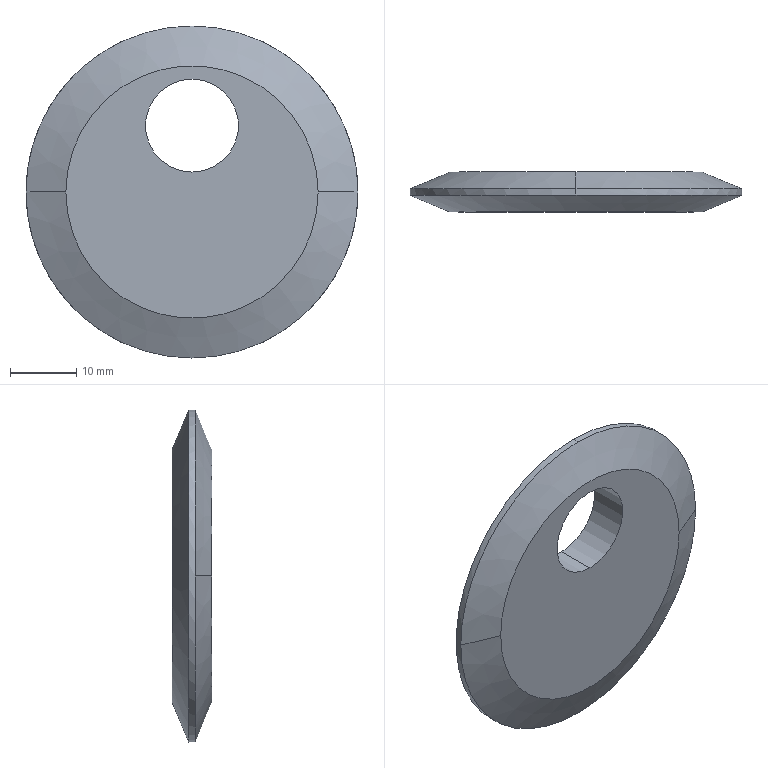Part | SolidWorks | features BaseBody 1 | 1 solid | 10 faces | box 50 x 6 x 50 mm | volume 8690 mm3 | cylinder 4 | cone 4 | plane 2 | commonest cylinder face diameters 14 x2 50 x2
STEP:
#1=CARTESIAN_POINT('',(57.247,561.007,-306.268));
#2=VERTEX_POINT('',#1);
#3=CARTESIAN_POINT('',(57.247,561.007,-292.268));
#4=VERTEX_POINT('',#3);
#5=CARTESIAN_POINT('',(57.247,561.007,-299.268));
#6=DIRECTION('',(0.,1.,0.));
#7=DIRECTION('',(0.,0.,1.));
#8=AXIS2_PLACEMENT_3D('',#5,#6,#7);
#9=CIRCLE('',#8,7.);
#10=EDGE_CURVE('',#2,#4,#9,.T.);
#11=ORIENTED_EDGE('',*,*,#10,.F.);
#12=CARTESIAN_POINT('',(57.247,567.007,-306.268));
#13=VERTEX_POINT('',#12);
#14=CARTESIAN_POINT('',(57.247,458.514,-306.268));
#15=DIRECTION('',(0.,1.,0.));
#16=VECTOR('',#15,1000.);
#17=LINE('',#14,#16);
#18=EDGE_CURVE('',#2,#13,#17,.T.);
#19=ORIENTED_EDGE('',*,*,#18,.T.);
#20=CARTESIAN_POINT('',(57.247,567.007,-292.268));
#21=VERTEX_POINT('',#20);
#22=CARTESIAN_POINT('',(57.247,567.007,-299.268));
#23=DIRECTION('',(0.,-1.,0.));
#24=DIRECTION('',(0.,0.,1.));
#25=AXIS2_PLACEMENT_3D('',#22,#23,#24);
#26=CIRCLE('',#25,7.);
#27=EDGE_CURVE('',#21,#13,#26,.T.);
#28=ORIENTED_EDGE('',*,*,#27,.F.);
#29=CARTESIAN_POINT('',(57.247,458.514,-292.268));
#30=DIRECTION('',(0.,1.,0.));
#31=VECTOR('',#30,1000.);
#32=LINE('',#29,#31);
#33=EDGE_CURVE('',#4,#21,#32,.T.);
#34=ORIENTED_EDGE('',*,*,#33,.F.);
#35=EDGE_LOOP('',(#11,#19,#28,#34));
#36=FACE_OUTER_BOUND('',#35,.T.);
#37=CARTESIAN_POINT('',(57.247,458.514,-299.268));
#38=DIRECTION('',(0.,1.,0.));
#39=DIRECTION('',(0.,0.,1.));
#40=AXIS2_PLACEMENT_3D('',#37,#38,#39);
#41=CYLINDRICAL_SURFACE('',#40,7.);
#42=ADVANCED_FACE('',(#36),#41,.F.);
#43=CARTESIAN_POINT('',(76.247,561.007,-309.268));
#44=VERTEX_POINT('',#43);
#45=CARTESIAN_POINT('',(38.247,561.007,-309.268));
#46=VERTEX_POINT('',#45);
#47=CARTESIAN_POINT('',(57.247,561.007,-309.268));
#48=DIRECTION('',(0.,-1.,0.));
#49=DIRECTION('',(-1.,0.,0.));
#50=AXIS2_PLACEMENT_3D('',#47,#48,#49);
#51=CIRCLE('',#50,19.);
#52=EDGE_CURVE('',#44,#46,#51,.T.);
#53=ORIENTED_EDGE('',*,*,#52,.F.);
#54=CARTESIAN_POINT('',(82.247,563.507,-309.268));
#55=VERTEX_POINT('',#54);
#56=CARTESIAN_POINT('',(82.247,563.507,-309.268));
#57=DIRECTION('',(0.9231,0.3846,0.));
#58=VECTOR('',#57,1000.);
#59=LINE('',#56,#58);
#60=EDGE_CURVE('',#44,#55,#59,.T.);
#61=ORIENTED_EDGE('',*,*,#60,.T.);
#62=CARTESIAN_POINT('',(57.247,563.507,-284.268));
#63=VERTEX_POINT('',#62);
#64=CARTESIAN_POINT('',(57.247,563.507,-309.268));
#65=DIRECTION('',(0.,-1.,0.));
#66=DIRECTION('',(0.,0.,1.));
#67=AXIS2_PLACEMENT_3D('',#64,#65,#66);
#68=CIRCLE('',#67,25.);
#69=EDGE_CURVE('',#55,#63,#68,.T.);
#70=ORIENTED_EDGE('',*,*,#69,.T.);
#71=CARTESIAN_POINT('',(32.247,563.507,-309.268));
#72=VERTEX_POINT('',#71);
#73=CARTESIAN_POINT('',(57.247,563.507,-309.268));
#74=DIRECTION('',(0.,-1.,0.));
#75=DIRECTION('',(0.,0.,1.));
#76=AXIS2_PLACEMENT_3D('',#73,#74,#75);
#77=CIRCLE('',#76,25.);
#78=EDGE_CURVE('',#63,#72,#77,.T.);
#79=ORIENTED_EDGE('',*,*,#78,.T.);
#80=CARTESIAN_POINT('',(32.247,563.507,-309.268));
#81=DIRECTION('',(-0.9231,0.3846,0.));
#82=VECTOR('',#81,1000.);
#83=LINE('',#80,#82);
#84=EDGE_CURVE('',#46,#72,#83,.T.);
#85=ORIENTED_EDGE('',*,*,#84,.F.);
#86=EDGE_LOOP('',(#53,#61,#70,#79,#85));
#87=FACE_OUTER_BOUND('',#86,.T.);
#88=CARTESIAN_POINT('',(57.247,563.507,-309.268));
#89=DIRECTION('',(0.,1.,0.));
#90=DIRECTION('',(-1.,0.,0.));
#91=AXIS2_PLACEMENT_3D('',#88,#89,#90);
#92=CONICAL_SURFACE('',#91,25.,1.176);
#93=ADVANCED_FACE('',(#87),#92,.T.);
#94=CARTESIAN_POINT('',(57.247,563.507,-334.268));
#95=VERTEX_POINT('',#94);
#96=CARTESIAN_POINT('',(57.247,563.507,-309.268));
#97=DIRECTION('',(0.,-1.,0.));
#98=DIRECTION('',(0.,0.,1.));
#99=AXIS2_PLACEMENT_3D('',#96,#97,#98);
#100=CIRCLE('',#99,25.);
#101=EDGE_CURVE('',#95,#55,#100,.T.);
#102=ORIENTED_EDGE('',*,*,#101,.F.);
#103=CARTESIAN_POINT('',(57.247,564.507,-334.268));
#104=VERTEX_POINT('',#103);
#105=CARTESIAN_POINT('',(57.247,561.007,-334.268));
#106=DIRECTION('',(0.,1.,0.));
#107=VECTOR('',#106,1000.);
#108=LINE('',#105,#107);
#109=EDGE_CURVE('',#95,#104,#108,.T.);
#110=ORIENTED_EDGE('',*,*,#109,.T.);
#111=CARTESIAN_POINT('',(57.247,564.507,-284.268));
#112=VERTEX_POINT('',#111);
#113=CARTESIAN_POINT('',(57.247,564.507,-309.268));
#114=DIRECTION('',(0.,-1.,0.));
#115=DIRECTION('',(0.,0.,1.));
#116=AXIS2_PLACEMENT_3D('',#113,#114,#115);
#117=CIRCLE('',#116,25.);
#118=EDGE_CURVE('',#104,#112,#117,.T.);
#119=ORIENTED_EDGE('',*,*,#118,.T.);
#120=CARTESIAN_POINT('',(57.247,561.007,-284.268));
#121=DIRECTION('',(0.,1.,0.));
#122=VECTOR('',#121,1000.);
#123=LINE('',#120,#122);
#124=EDGE_CURVE('',#63,#112,#123,.T.);
#125=ORIENTED_EDGE('',*,*,#124,.F.);
#126=ORIENTED_EDGE('',*,*,#69,.F.);
#127=EDGE_LOOP('',(#102,#110,#119,#125,#126));
#128=FACE_OUTER_BOUND('',#127,.T.);
#129=CARTESIAN_POINT('',(57.247,561.007,-309.268));
#130=DIRECTION('',(0.,1.,0.));
#131=DIRECTION('',(0.,0.,1.));
#132=AXIS2_PLACEMENT_3D('',#129,#130,#131);
#133=CYLINDRICAL_SURFACE('',#132,25.);
#134=ADVANCED_FACE('',(#128),#133,.T.);
#135=CARTESIAN_POINT('',(57.247,567.007,-290.268));
#136=VERTEX_POINT('',#135);
#137=CARTESIAN_POINT('',(57.247,567.007,-328.268));
#138=VERTEX_POINT('',#137);
#139=CARTESIAN_POINT('',(57.247,567.007,-309.268));
#140=DIRECTION('',(0.,1.,0.));
#141=DIRECTION('',(0.,0.,-1.));
#142=AXIS2_PLACEMENT_3D('',#139,#140,#141);
#143=CIRCLE('',#142,19.);
#144=EDGE_CURVE('',#136,#138,#143,.T.);
#145=ORIENTED_EDGE('',*,*,#144,.F.);
#146=CARTESIAN_POINT('',(57.247,564.507,-284.268));
#147=DIRECTION('',(0.,-0.3846,0.9231));
#148=VECTOR('',#147,1000.);
#149=LINE('',#146,#148);
#150=EDGE_CURVE('',#136,#112,#149,.T.);
#151=ORIENTED_EDGE('',*,*,#150,.T.);
#152=ORIENTED_EDGE('',*,*,#118,.F.);
#153=CARTESIAN_POINT('',(57.247,564.507,-334.268));
#154=DIRECTION('',(0.,-0.3846,-0.9231));
#155=VECTOR('',#154,1000.);
#156=LINE('',#153,#155);
#157=EDGE_CURVE('',#138,#104,#156,.T.);
#158=ORIENTED_EDGE('',*,*,#157,.F.);
#159=EDGE_LOOP('',(#145,#151,#152,#158));
#160=FACE_OUTER_BOUND('',#159,.T.);
#161=CARTESIAN_POINT('',(57.247,564.507,-309.268));
#162=DIRECTION('',(0.,-1.,0.));
#163=DIRECTION('',(0.,0.,-1.));
#164=AXIS2_PLACEMENT_3D('',#161,#162,#163);
#165=CONICAL_SURFACE('',#164,25.,1.176);
#166=ADVANCED_FACE('',(#160),#165,.T.);
#167=CARTESIAN_POINT('',(57.247,561.007,-299.268));
#168=DIRECTION('',(0.,1.,0.));
#169=DIRECTION('',(0.,0.,1.));
#170=AXIS2_PLACEMENT_3D('',#167,#168,#169);
#171=CIRCLE('',#170,7.);
#172=EDGE_CURVE('',#4,#2,#171,.T.);
#173=ORIENTED_EDGE('',*,*,#172,.T.);
#174=ORIENTED_EDGE('',*,*,#10,.T.);
#175=EDGE_LOOP('',(#173,#174));
#176=FACE_BOUND('',#175,.T.);
#177=CARTESIAN_POINT('',(57.247,561.007,-309.268));
#178=DIRECTION('',(0.,-1.,0.));
#179=DIRECTION('',(-1.,0.,0.));
#180=AXIS2_PLACEMENT_3D('',#177,#178,#179);
#181=CIRCLE('',#180,19.);
#182=EDGE_CURVE('',#46,#44,#181,.T.);
#183=ORIENTED_EDGE('',*,*,#182,.T.);
#184=ORIENTED_EDGE('',*,*,#52,.T.);
#185=EDGE_LOOP('',(#183,#184));
#186=FACE_OUTER_BOUND('',#185,.T.);
#187=CARTESIAN_POINT('',(57.247,561.007,-309.268));
#188=DIRECTION('',(0.,-1.,0.));
#189=DIRECTION('',(0.,0.,-1.));
#190=AXIS2_PLACEMENT_3D('',#187,#188,#189);
#191=PLANE('',#190);
#192=ADVANCED_FACE('',(#176,#186),#191,.T.);
#193=ORIENTED_EDGE('',*,*,#18,.F.);
#194=ORIENTED_EDGE('',*,*,#172,.F.);
#195=ORIENTED_EDGE('',*,*,#33,.T.);
#196=CARTESIAN_POINT('',(57.247,567.007,-299.268));
#197=DIRECTION('',(0.,-1.,0.));
#198=DIRECTION('',(0.,0.,1.));
#199=AXIS2_PLACEMENT_3D('',#196,#197,#198);
#200=CIRCLE('',#199,7.);
#201=EDGE_CURVE('',#13,#21,#200,.T.);
#202=ORIENTED_EDGE('',*,*,#201,.F.);
#203=EDGE_LOOP('',(#193,#194,#195,#202));
#204=FACE_OUTER_BOUND('',#203,.T.);
#205=CARTESIAN_POINT('',(57.247,458.514,-299.268));
#206=DIRECTION('',(0.,1.,0.));
#207=DIRECTION('',(0.,0.,1.));
#208=AXIS2_PLACEMENT_3D('',#205,#206,#207);
#209=CYLINDRICAL_SURFACE('',#208,7.);
#210=ADVANCED_FACE('',(#204),#209,.F.);
#211=ORIENTED_EDGE('',*,*,#60,.F.);
#212=ORIENTED_EDGE('',*,*,#182,.F.);
#213=ORIENTED_EDGE('',*,*,#84,.T.);
#214=CARTESIAN_POINT('',(57.247,563.507,-309.268));
#215=DIRECTION('',(0.,-1.,0.));
#216=DIRECTION('',(0.,0.,1.));
#217=AXIS2_PLACEMENT_3D('',#214,#215,#216);
#218=CIRCLE('',#217,25.);
#219=EDGE_CURVE('',#72,#95,#218,.T.);
#220=ORIENTED_EDGE('',*,*,#219,.T.);
#221=ORIENTED_EDGE('',*,*,#101,.T.);
#222=EDGE_LOOP('',(#211,#212,#213,#220,#221));
#223=FACE_OUTER_BOUND('',#222,.T.);
#224=CARTESIAN_POINT('',(57.247,563.507,-309.268));
#225=DIRECTION('',(0.,1.,0.));
#226=DIRECTION('',(-1.,0.,0.));
#227=AXIS2_PLACEMENT_3D('',#224,#225,#226);
#228=CONICAL_SURFACE('',#227,25.,1.176);
#229=ADVANCED_FACE('',(#223),#228,.T.);
#230=ORIENTED_EDGE('',*,*,#27,.T.);
#231=ORIENTED_EDGE('',*,*,#201,.T.);
#232=EDGE_LOOP('',(#230,#231));
#233=FACE_BOUND('',#232,.T.);
#234=CARTESIAN_POINT('',(57.247,567.007,-309.268));
#235=DIRECTION('',(0.,1.,0.));
#236=DIRECTION('',(0.,0.,-1.));
#237=AXIS2_PLACEMENT_3D('',#234,#235,#236);
#238=CIRCLE('',#237,19.);
#239=EDGE_CURVE('',#138,#136,#238,.T.);
#240=ORIENTED_EDGE('',*,*,#239,.T.);
#241=ORIENTED_EDGE('',*,*,#144,.T.);
#242=EDGE_LOOP('',(#240,#241));
#243=FACE_OUTER_BOUND('',#242,.T.);
#244=CARTESIAN_POINT('',(57.247,567.007,-309.268));
#245=DIRECTION('',(0.,1.,0.));
#246=DIRECTION('',(0.,0.,1.));
#247=AXIS2_PLACEMENT_3D('',#244,#245,#246);
#248=PLANE('',#247);
#249=ADVANCED_FACE('',(#233,#243),#248,.T.);
#250=ORIENTED_EDGE('',*,*,#109,.F.);
#251=ORIENTED_EDGE('',*,*,#219,.F.);
#252=ORIENTED_EDGE('',*,*,#78,.F.);
#253=ORIENTED_EDGE('',*,*,#124,.T.);
#254=CARTESIAN_POINT('',(57.247,564.507,-309.268));
#255=DIRECTION('',(0.,-1.,0.));
#256=DIRECTION('',(0.,0.,1.));
#257=AXIS2_PLACEMENT_3D('',#254,#255,#256);
#258=CIRCLE('',#257,25.);
#259=EDGE_CURVE('',#112,#104,#258,.T.);
#260=ORIENTED_EDGE('',*,*,#259,.T.);
#261=EDGE_LOOP('',(#250,#251,#252,#253,#260));
#262=FACE_OUTER_BOUND('',#261,.T.);
#263=CARTESIAN_POINT('',(57.247,561.007,-309.268));
#264=DIRECTION('',(0.,1.,0.));
#265=DIRECTION('',(0.,0.,1.));
#266=AXIS2_PLACEMENT_3D('',#263,#264,#265);
#267=CYLINDRICAL_SURFACE('',#266,25.);
#268=ADVANCED_FACE('',(#262),#267,.T.);
#269=ORIENTED_EDGE('',*,*,#150,.F.);
#270=ORIENTED_EDGE('',*,*,#239,.F.);
#271=ORIENTED_EDGE('',*,*,#157,.T.);
#272=ORIENTED_EDGE('',*,*,#259,.F.);
#273=EDGE_LOOP('',(#269,#270,#271,#272));
#274=FACE_OUTER_BOUND('',#273,.T.);
#275=CARTESIAN_POINT('',(57.247,564.507,-309.268));
#276=DIRECTION('',(0.,-1.,0.));
#277=DIRECTION('',(0.,0.,-1.));
#278=AXIS2_PLACEMENT_3D('',#275,#276,#277);
#279=CONICAL_SURFACE('',#278,25.,1.176);
#280=ADVANCED_FACE('',(#274),#279,.T.);
#281=CLOSED_SHELL('',(#42,#93,#134,#166,#192,#210,#229,#249,#268,#280));
#282=MANIFOLD_SOLID_BREP('',#281);
#283=CARTESIAN_POINT('',(0.,0.,0.));
#284=DIRECTION('',(0.,0.,1.));
#285=DIRECTION('',(1.,0.,0.));
#286=AXIS2_PLACEMENT_3D('',#283,#284,#285);
#287=(LENGTH_UNIT()NAMED_UNIT(*)SI_UNIT(.MILLI.,.METRE.));
#288=UNCERTAINTY_MEASURE_WITH_UNIT(LENGTH_MEASURE(0.00001),#287,'','');
#289=(NAMED_UNIT(*)PLANE_ANGLE_UNIT()SI_UNIT($,.RADIAN.));
#290=(NAMED_UNIT(*)SI_UNIT($,.STERADIAN.)SOLID_ANGLE_UNIT());
#291=(GEOMETRIC_REPRESENTATION_CONTEXT(3)GLOBAL_UNCERTAINTY_ASSIGNED_CONTEXT((#288))GLOBAL_UNIT_ASSIGNED_CONTEXT((#287,#289,#290))REPRESENTATION_CONTEXT('',''));
#292=ADVANCED_BREP_SHAPE_REPRESENTATION('',(#282,#286),#291);